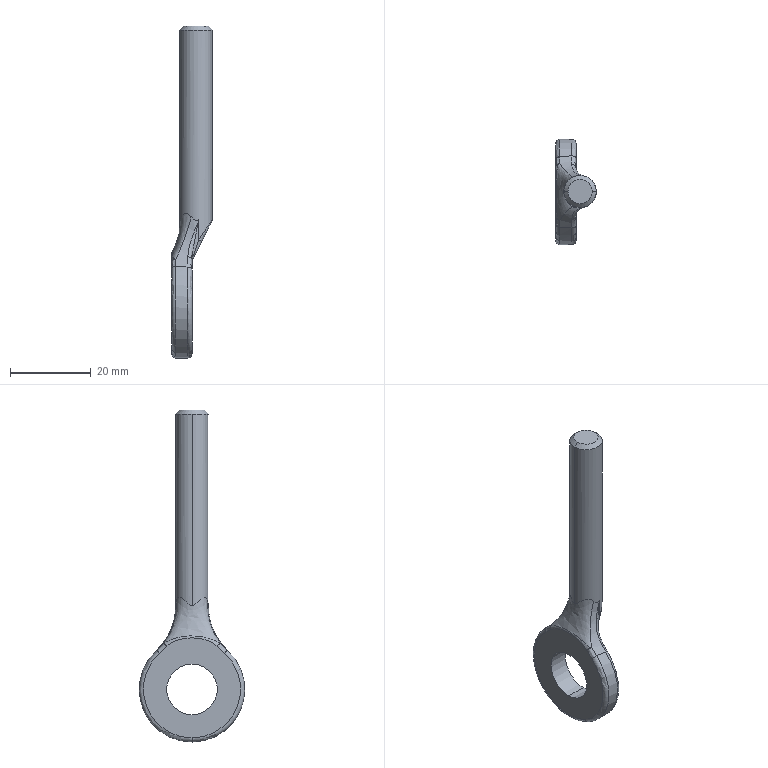Part | SolidWorks | features BaseBody 1 | 1 solid | 37 faces | box 10 x 26 x 82 mm | volume 4881 mm3 | spline 18 | cylinder 9 | torus 4 | plane 4 | cone 2 | commonest cylinder face diameters 4 x2 8 x2 12.5 x2 26 x2 2 x1